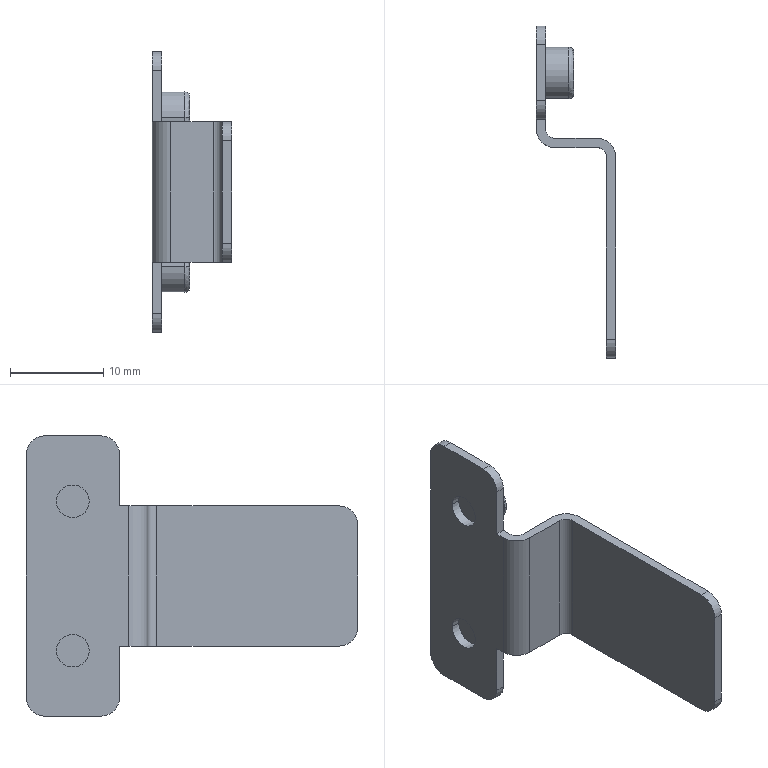Part | SolidWorks | features BaseBody 1 | 1 solid | 54 faces | box 8.5 x 35.5 x 30 mm | volume 877.993 mm3 | plane 32 | cylinder 18 | spline 4 | commonest cylinder face diameters 4 x8 3.5 x4 5.5 x4 2 x2